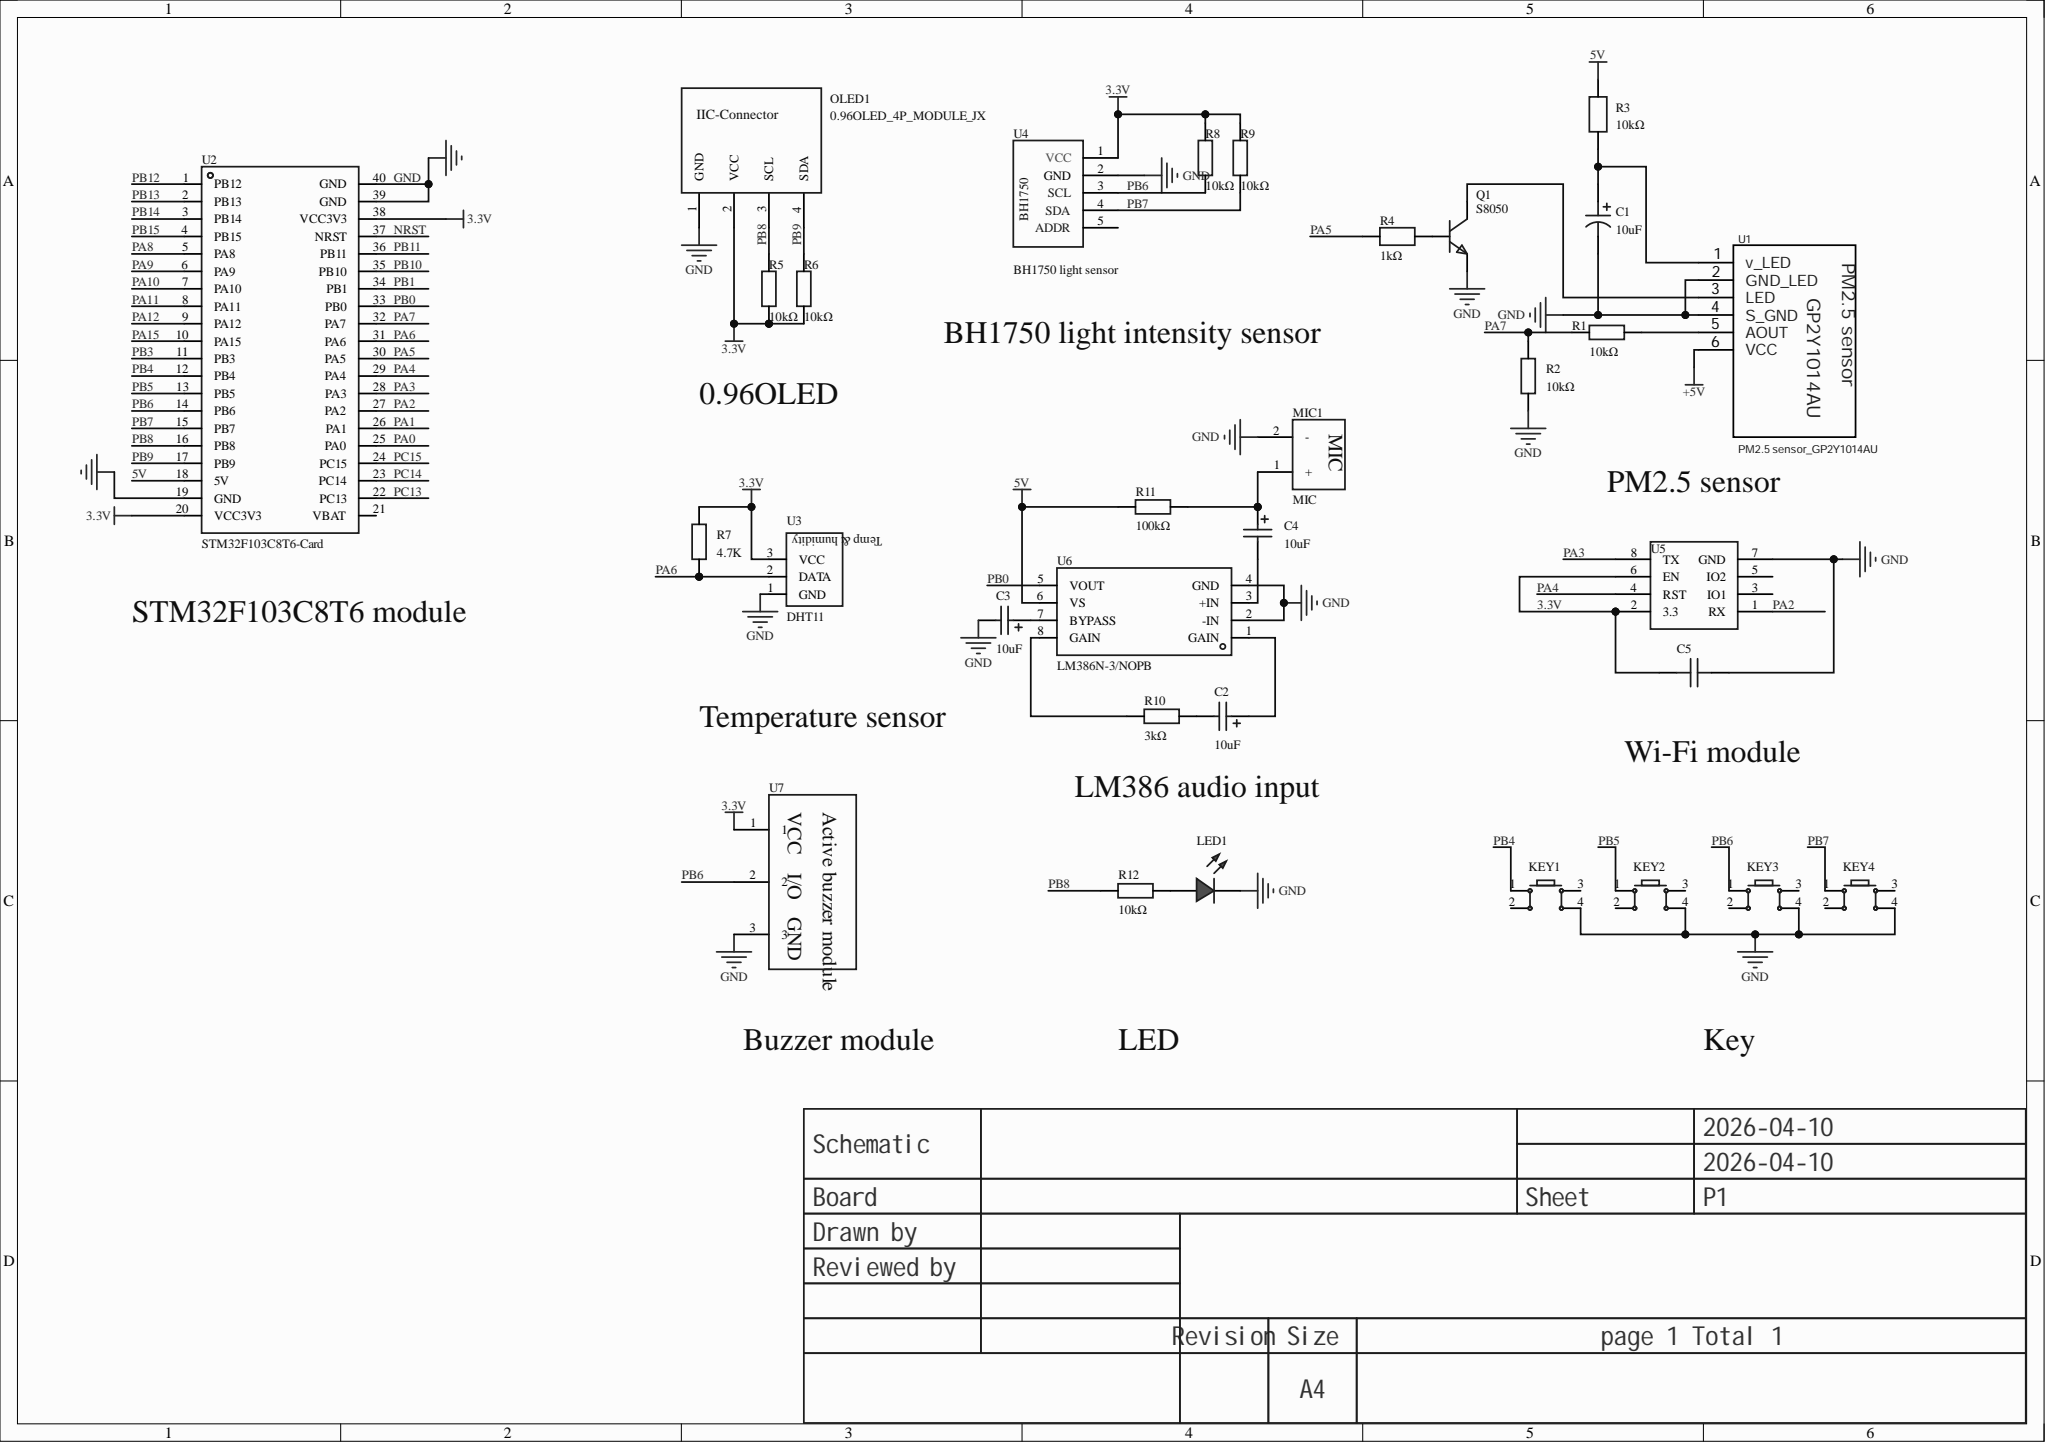Circuit board | Altium Designer | 32 parts | 27 nets
Bill of materials:
Comment,Description,Designator,Footprint,LibRef,Quantity
"10uF","Capacitance:10uF;Tolerance:±20%;Rated voltage:63V;","C1","CAP-TH_BD5.0-P2.00-D0.5-FD","SHG63V10UF03EC0822","1"
"10uF","","C2, C3, C4","C_Ele_SMD_3x5.4mm","C_Ele_SMD_3x5.4mm","3"
"5pF","Capacitance:5pF;Rated voltage:50V;Temp coefficient:COH;","C5","CAP-TH_L5.0-W3.0-P5.00-D0.6","DCC509D20COHF6FJ5A0","1"
"","","KEY1, KEY2, KEY3, KEY4","SW-TH_4P-L6.0-W6.0-P4.50-LS6.5","Key_TH_6x6x6","4"
"","","LED1","LED_TH-3mm","LED_TH-R_3mm","1"
"MIC","","MIC1","MIC-TH_BD6.0-P2.00","MIC","1"
"0.96OLED_4P_MODULE_JX","","OLED1","0.96OLED_4P","0.96OLED_4P_MODULE_JX","1"
"S8050","Transistor type:NPN;Collector current(Ic):500mA;Collector-emitter breakdown voltage(Vceo):25V;Power dissipation(Pd):625mW;DC current gain(hFE):160@50mA,1V;","Q1","TO-92-3_L4.5-W3.5-P1.27-L","S8050_C2931492","1"
"10kΩ","","R1, R2, R5, R6, R8, R9, R12","Res_1/4W","Res_AXIAL-1/4W","7"
"10kΩ","Resistor type:metal film resistor;Resistance:10kΩ;Tolerance:±1%;Power:250mW;Temp coefficient:±100ppm/?;","R3","RES-TH_BD2.7-L6.2-P10.20-D0.4","MF1/4W-10K±1%-ST52","1"
"1kΩ","Resistor type:metal film resistor;Resistance:1kΩ;Tolerance:±1%;Power:250mW;Temp coefficient:±100ppm/?;","R4","RES-TH_BD2.7-L6.2-P10.20-D0.4","MF1/4W-1K±1%-ST52","1"
"4.7K","","R7","Res_1/4W","Res_AXIAL-1/4W","1"
"3kΩ","","R10","Res_1/4W","Res_AXIAL-1/4W","1"
"100kΩ","","R11","Res_1/4W","Res_AXIAL-1/4W","1"
"PM2.5 sensor_GP2Y1014AU","","U1","PM2.5传感器_GP2Y1014AU","PM2.5传感器_GP2Y1014AU","1"
"STM32F103C8T6-Card","","U2","CONN-TH_L53.3-W22.9_STM32F103C8T6-CARD","STM32F103C8T6-Card","1"
"DHT11","","U3","DHT11","DHT11","1"
"","","U4","BH1750光照传感器","BH1750光照传感器","1"
"","esp8266 module pinout diagram","U5","ESP8266-1","esp8266","1"
"LM386N-3/NOPB","Amplifier type:class AB;Speaker channels:mono;Output power:700mWx1@8Ω;Quiescent current(Iq):4mA;","U6","DIP-8_L9.8-W6.6-P2.54-LS7.6-BL","LM386N-3/NOPB","1"
"","","U7","有源蜂鸣器模块","有源蜂鸣器模块","1"
Netlist (Protel format):
[
C1
CAP-TH_BD5.0-P2.00-D0.5-FD
10uF



]
[
C2
C_Ele_SMD_3x5.4mm
10uF



]
[
C3
C_Ele_SMD_3x5.4mm
10uF



]
[
C4
C_Ele_SMD_3x5.4mm
10uF



]
[
C5
CAP-TH_L5.0-W3.0-P5.00-D0.6
5pF



]
[
KEY1
SW-TH_4P-L6.0-W6.0-P4.50-LS6.5




]
[
KEY2
SW-TH_4P-L6.0-W6.0-P4.50-LS6.5




]
[
KEY3
SW-TH_4P-L6.0-W6.0-P4.50-LS6.5




]
[
KEY4
SW-TH_4P-L6.0-W6.0-P4.50-LS6.5




]
[
LED1
LED_TH-3mm




]
[
MIC1
MIC-TH_BD6.0-P2.00
MIC



]
[
OLED1
0.96OLED_4P
0.96OLED_4P_MODULE_JX



]
[
Q1
TO-92-3_L4.5-W3.5-P1.27-L
S8050



]
[
R1
Res_1/4W
10kΩ



]
[
R2
Res_1/4W
10kΩ



]
[
R3
RES-TH_BD2.7-L6.2-P10.20-D0.4
10kΩ



]
[
R4
RES-TH_BD2.7-L6.2-P10.20-D0.4
1kΩ



]
[
R5
Res_1/4W
10kΩ



]
[
R6
Res_1/4W
10kΩ



]
[
R7
Res_1/4W
4.7K



]
[
R8
Res_1/4W
10kΩ



]
[
R9
Res_1/4W
10kΩ



]
[
R10
Res_1/4W
3kΩ



]
[
R11
Res_1/4W
100kΩ



]
[
R12
Res_1/4W
10kΩ



]
[
U1
PM2.5传感器_GP2Y1014AU
PM2.5 sensor_GP2Y1014AU



]
[
U2
CONN-TH_L53.3-W22.9_STM32F103C8T6-CARD
STM32F103C8T6-Card



]
[
U3
DHT11
DHT11



]
[
U4
BH1750光照传感器




]
[
U5
ESP8266-1




]
[
U6
DIP-8_L9.8-W6.6-P2.54-LS7.6-BL
LM386N-3/NOPB



]
[
U7
有源蜂鸣器模块




]
(
PB9
OLED1-4
R6-2
U2-17
)
(
PB8
OLED1-3
R5-2
R12-2
U2-16
)
(
PB7
KEY4-1
R9-1
U2-15
U4-4
)
(
PB6
KEY3-1
R8-1
U2-14
U4-3
U7-2
)
(
PB5
KEY2-1
U2-13
)
(
PB4
KEY1-1
U2-12
)
(
PB0
U2-33
U6-5
)
(
PA7
R1-1
R2-2
U2-32
)
(
PA6
R7-1
U2-31
U3-2
)
(
PA5
R4-1
U2-30
)
(
PA4
U2-29
U5-4
)
(
PA3
U2-28
U5-8
)
(
PA2
U2-27
U5-1
)
(
NetR10_1
R10-1
U6-8
)
(
NetR1_2
R1-2
U1-5
)
(
NetQ1_3
Q1-3
U1-3
)
(
NetQ1_2
Q1-2
R4-2
)
(
NetLED1_1
LED1-1
R12-1
)
(
NetC4_2
C4-2
U6-3
)
(
NetC4_1
C4-1
MIC1-1
R11-2
)
(
NetC3_1
C3-1
U6-7
)
(
NetC2_2
C2-2
R10-2
)
(
NetC2_1
C2-1
U6-1
)
(
NetC1_1
C1-1
R3-1
U1-1
)
(
GND
C1-2
C3-2
C5-2
KEY1-4
KEY2-4
KEY3-4
KEY4-4
LED1-2
MIC1-2
OLED1-1
Q1-1
R2-1
U1-2
U1-4
U2-19
U2-39
U2-40
U3-1
U4-2
U5-7
U6-2
U6-4
U7-3
)
(
5V
R3-2
R11-1
U2-18
U6-6
)
(
3.3V
C5-1
OLED1-2
R5-1
R6-1
R7-2
R8-2
R9-2
U2-20
U2-38
U3-3
U4-1
U5-2
U5-6
U7-1
)